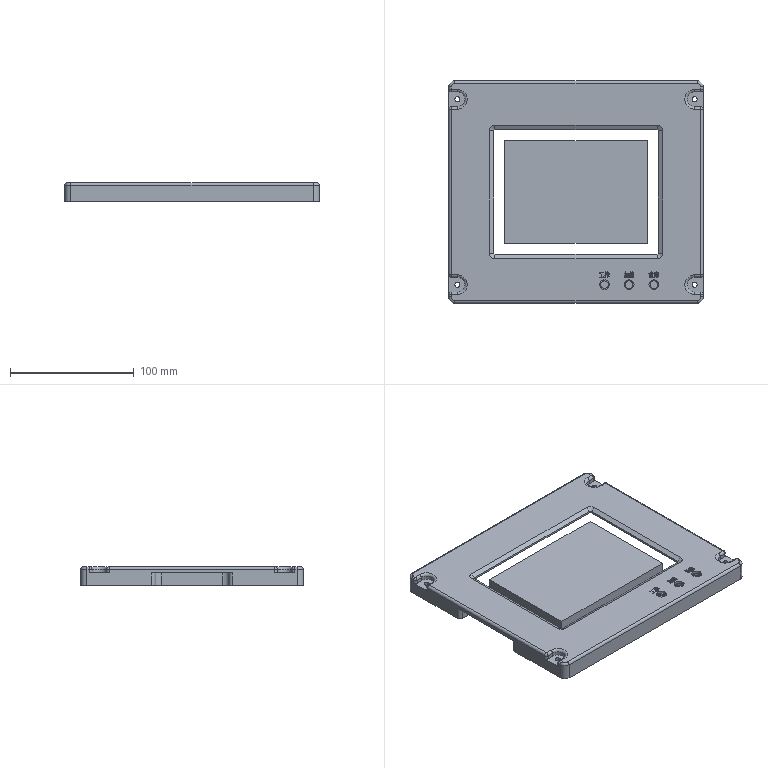NC program | Mastercam | posted with a generic post | part box 206 x 180 x 15 mm
Lines 17302 to 18142 of 42274:
(4 FEM |TOOL - 4|DIA. OFF. - 4|LEN. - 4|TOOL DIA. - 4.)
N4968 T4 M6
N4970 G0 G54 G90 X23. Y-75. C0. B0. S10000 M3
N4972 G43 H4 Z50.
N4974 Z1.
N4976 G1 Z0. F600.
N4978 X21.695 Y-74.65 F3000.
N4980 G3 X21.217 Y-75.478 I.478 J-.828
N4982 X21.346 Y-75.955 I.956
N4984 X23. Y-76.91 Z-.05 I1.654 J.955
N4986 X24.91 Y-75. Z-.125 J1.91
N4988 X23. Y-73.09 Z-.2 I-1.91
N4990 X21.09 Y-75. Z-.275 J-1.91
N4992 X21.346 Y-75.955 Z-.3 I1.91
N4994 X23. Y-76.91 Z-.35 I1.654 J.955
N4996 X24.91 Y-75. Z-.425 J1.91
N4998 X23. Y-73.09 Z-.5 I-1.91
N5000 X21.09 Y-75. Z-.575 J-1.91
N5002 X21.346 Y-75.955 Z-.6 I1.91
N5004 X23. Y-76.91 Z-.65 I1.654 J.955
N5006 X24.91 Y-75. Z-.725 J1.91
N5008 X23. Y-73.09 Z-.8 I-1.91
N5010 X21.09 Y-75. Z-.875 J-1.91
N5012 X21.346 Y-75.955 Z-.9 I1.91
N5014 X23. Y-76.91 Z-.95 I1.654 J.955
N5016 X24.91 Y-75. Z-1.025 J1.91
N5018 X23. Y-73.09 Z-1.1 I-1.91
N5020 X21.09 Y-75. Z-1.175 J-1.91
N5022 X21.346 Y-75.955 Z-1.2 I1.91
N5024 X23. Y-76.91 Z-1.25 I1.654 J.955
N5026 X24.91 Y-75. Z-1.325 J1.91
N5028 X23. Y-73.09 Z-1.4 I-1.91
N5030 X21.09 Y-75. Z-1.475 J-1.91
N5032 X21.346 Y-75.955 Z-1.5 I1.91
N5034 X23. Y-76.91 Z-1.55 I1.654 J.955
N5036 X24.91 Y-75. Z-1.625 J1.91
N5038 X23. Y-73.09 Z-1.7 I-1.91
N5040 X21.09 Y-75. Z-1.775 J-1.91
N5042 X21.346 Y-75.955 Z-1.8 I1.91
N5044 X23. Y-76.91 Z-1.85 I1.654 J.955
N5046 X24.91 Y-75. Z-1.925 J1.91
N5048 X23. Y-73.09 Z-2. I-1.91
N5050 X21.09 Y-75. J-1.91 F1500.
N5052 X23. Y-76.91 I1.91
N5054 X24.91 Y-75. J1.91
N5056 X23. Y-73.09 I-1.91
N5058 X22.506 Y-73.155 J-1.91
N5060 X21.798 Y-74.078 I.247 J-.923
N5062 X21.83 Y-74.325 I.955
N5064 G1 X23. Y-75.
N5066 G0 Z0.
N5068 G1 X24.005 Y-73.995 F750.
N5070 G3 X23. Y-72.99 I-1.005
N5072 X20.99 Y-75. J-2.01
N5074 X23. Y-77.01 I2.01
N5076 X25.01 Y-75. J2.01
N5078 X23. Y-72.99 I-2.01
N5080 X22.505 Y-73.052 J-2.01
N5082 X20.99 Y-75. Z-.631 I.495 J-1.948
N5084 X23. Y-77.01 Z-1.381 I2.01
N5086 X24.935 Y-75.546 Z-2. J2.01
N5088 X25.011 Y-75. I-1.935 J.546
N5090 X23. Y-72.989 I-2.011
N5092 X20.989 Y-75. J-2.011
N5094 X23. Y-77.011 I2.011
N5096 X24.935 Y-75.546 J2.011
N5098 X25.009 Y-75.052 I-1.935 J.546
N5100 G1 Y-75.026
N5102 G3 X24.031 Y-74.022 I-1.004
N5104 G1 X23. Y-75.
N5106 G0 Z50.
N5108 Z48.
N5110 Z-1.
N5112 G1 Z-2. F600.
N5114 X23.505 Y-74.495 F3000.
N5116 G3 X23. Y-73.99 I-.505
N5118 X21.99 Y-75. Z-2.075 J-1.01
N5120 X23. Y-76.01 Z-2.15 I1.01
N5122 X24.01 Y-75. Z-2.225 J1.01
N5124 X23. Y-73.99 Z-2.3 I-1.01
N5126 X21.99 Y-75. Z-2.375 J-1.01
N5128 X23. Y-76.01 Z-2.45 I1.01
N5130 X24.01 Y-75. Z-2.525 J1.01
N5132 X23. Y-73.99 Z-2.6 I-1.01
N5134 X21.99 Y-75. Z-2.675 J-1.01
N5136 X23. Y-76.01 Z-2.75 I1.01
N5138 X24.01 Y-75. Z-2.825 J1.01
N5140 X23. Y-73.99 Z-2.9 I-1.01
N5142 X21.99 Y-75. Z-2.975 J-1.01
N5144 X23. Y-76.01 Z-3.05 I1.01
N5146 X24.01 Y-75. Z-3.125 J1.01
N5148 X23. Y-73.99 Z-3.2 I-1.01
N5150 X21.99 Y-75. Z-3.275 J-1.01
N5152 X23. Y-76.01 Z-3.35 I1.01
N5154 X24.01 Y-75. Z-3.425 J1.01
N5156 X23. Y-73.99 Z-3.5 I-1.01
N5158 X21.99 Y-75. J-1.01 F1500.
N5160 X23. Y-76.01 I1.01
N5162 X24.01 Y-75. J1.01
N5164 X23. Y-73.99 I-1.01
N5166 X22.52 Y-74.111 J-1.01
N5168 X22.254 Y-74.556 I.24 J-.445
N5170 X22.316 Y-74.796 I.506
N5172 G1 X23. Y-75.
N5174 G0 Z-2.
N5176 G1 X23.555 Y-74.445 F750.
N5178 G3 X23. Y-73.89 I-.555
N5180 X21.89 Y-75. J-1.11
N5182 X23. Y-76.11 I1.11
N5184 X24.11 Y-75. J1.11
N5186 X23. Y-73.89 I-1.11
N5188 X22.517 Y-74.001 J-1.11
N5190 X21.89 Y-75. Z-2.535 I.483 J-.999
N5192 X23. Y-76.11 Z-3.285 I1.11
N5194 X23.483 Y-75.999 Z-3.5 J1.11
N5196 X24.11 Y-75. I-.483 J.999
N5198 X23. Y-73.89 I-1.11
N5200 X21.89 Y-75. J-1.11
N5202 X23. Y-76.11 I1.11
N5204 X23.483 Y-75.999 J1.11
N5206 X23.87 Y-75.689 I-.483 J.999
N5208 X23.99 Y-75.345 I-.435 J.344
N5210 X23.78 Y-74.91 I-.555
N5212 G1 X23. Y-75.
N5214 G0 Z48.
N5216 Z50.
N5218 X43.
N5220 Z1.
N5222 G1 Z0. F600.
N5224 X41.695 Y-74.65 F3000.
N5226 G3 X41.217 Y-75.478 I.478 J-.828
N5228 X41.346 Y-75.955 I.956
N5230 X43. Y-76.91 Z-.05 I1.654 J.955
N5232 X44.91 Y-75. Z-.125 J1.91
N5234 X43. Y-73.09 Z-.2 I-1.91
N5236 X41.09 Y-75. Z-.275 J-1.91
N5238 X41.346 Y-75.955 Z-.3 I1.91
N5240 X43. Y-76.91 Z-.35 I1.654 J.955
N5242 X44.91 Y-75. Z-.425 J1.91
N5244 X43. Y-73.09 Z-.5 I-1.91
N5246 X41.09 Y-75. Z-.575 J-1.91
N5248 X41.346 Y-75.955 Z-.6 I1.91
N5250 X43. Y-76.91 Z-.65 I1.654 J.955
N5252 X44.91 Y-75. Z-.725 J1.91
N5254 X43. Y-73.09 Z-.8 I-1.91
N5256 X41.09 Y-75. Z-.875 J-1.91
N5258 X41.346 Y-75.955 Z-.9 I1.91
N5260 X43. Y-76.91 Z-.95 I1.654 J.955
N5262 X44.91 Y-75. Z-1.025 J1.91
N5264 X43. Y-73.09 Z-1.1 I-1.91
N5266 X41.09 Y-75. Z-1.175 J-1.91
N5268 X41.346 Y-75.955 Z-1.2 I1.91
N5270 X43. Y-76.91 Z-1.25 I1.654 J.955
N5272 X44.91 Y-75. Z-1.325 J1.91
N5274 X43. Y-73.09 Z-1.4 I-1.91
N5276 X41.09 Y-75. Z-1.475 J-1.91
N5278 X41.346 Y-75.955 Z-1.5 I1.91
N5280 X43. Y-76.91 Z-1.55 I1.654 J.955
N5282 X44.91 Y-75. Z-1.625 J1.91
N5284 X43. Y-73.09 Z-1.7 I-1.91
N5286 X41.09 Y-75. Z-1.775 J-1.91
N5288 X41.346 Y-75.955 Z-1.8 I1.91
N5290 X43. Y-76.91 Z-1.85 I1.654 J.955
N5292 X44.91 Y-75. Z-1.925 J1.91
N5294 X43. Y-73.09 Z-2. I-1.91
N5296 X41.09 Y-75. J-1.91 F1500.
N5298 X43. Y-76.91 I1.91
N5300 X44.91 Y-75. J1.91
N5302 X43. Y-73.09 I-1.91
N5304 X42.506 Y-73.155 J-1.91
N5306 X41.798 Y-74.078 I.247 J-.923
N5308 X41.83 Y-74.325 I.955
N5310 G1 X43. Y-75.
N5312 G0 Z0.
N5314 G1 X44.005 Y-73.995 F750.
N5316 G3 X43. Y-72.99 I-1.005
N5318 X40.99 Y-75. J-2.01
N5320 X43. Y-77.01 I2.01
N5322 X45.01 Y-75. J2.01
N5324 X43. Y-72.99 I-2.01
N5326 X42.505 Y-73.052 J-2.01
N5328 X40.99 Y-75. Z-.631 I.495 J-1.948
N5330 X43. Y-77.01 Z-1.381 I2.01
N5332 X44.935 Y-75.546 Z-2. J2.01
N5334 X45.011 Y-75. I-1.935 J.546
N5336 X43. Y-72.989 I-2.011
N5338 X40.989 Y-75. J-2.011
N5340 X43. Y-77.011 I2.011
N5342 X44.935 Y-75.546 J2.011
N5344 X45.009 Y-75.052 I-1.935 J.546
N5346 G1 Y-75.026
N5348 G3 X44.031 Y-74.022 I-1.004
N5350 G1 X43. Y-75.
N5352 G0 Z50.
N5354 Z48.
N5356 Z-1.
N5358 G1 Z-2. F600.
N5360 X43.505 Y-74.495 F3000.
N5362 G3 X43. Y-73.99 I-.505
N5364 X41.99 Y-75. Z-2.075 J-1.01
N5366 X43. Y-76.01 Z-2.15 I1.01
N5368 X44.01 Y-75. Z-2.225 J1.01
N5370 X43. Y-73.99 Z-2.3 I-1.01
N5372 X41.99 Y-75. Z-2.375 J-1.01
N5374 X43. Y-76.01 Z-2.45 I1.01
N5376 X44.01 Y-75. Z-2.525 J1.01
N5378 X43. Y-73.99 Z-2.6 I-1.01
N5380 X41.99 Y-75. Z-2.675 J-1.01
N5382 X43. Y-76.01 Z-2.75 I1.01
N5384 X44.01 Y-75. Z-2.825 J1.01
N5386 X43. Y-73.99 Z-2.9 I-1.01
N5388 X41.99 Y-75. Z-2.975 J-1.01
N5390 X43. Y-76.01 Z-3.05 I1.01
N5392 X44.01 Y-75. Z-3.125 J1.01
N5394 X43. Y-73.99 Z-3.2 I-1.01
N5396 X41.99 Y-75. Z-3.275 J-1.01
N5398 X43. Y-76.01 Z-3.35 I1.01
N5400 X44.01 Y-75. Z-3.425 J1.01
N5402 X43. Y-73.99 Z-3.5 I-1.01
N5404 X41.99 Y-75. J-1.01 F1500.
N5406 X43. Y-76.01 I1.01
N5408 X44.01 Y-75. J1.01
N5410 X43. Y-73.99 I-1.01
N5412 X42.52 Y-74.111 J-1.01
N5414 X42.254 Y-74.556 I.24 J-.445
N5416 X42.316 Y-74.796 I.506
N5418 G1 X43. Y-75.
N5420 G0 Z-2.
N5422 G1 X43.555 Y-74.445 F750.
N5424 G3 X43. Y-73.89 I-.555
N5426 X41.89 Y-75. J-1.11
N5428 X43. Y-76.11 I1.11
N5430 X44.11 Y-75. J1.11
N5432 X43. Y-73.89 I-1.11
N5434 X42.517 Y-74.001 J-1.11
N5436 X41.89 Y-75. Z-2.535 I.483 J-.999
N5438 X43. Y-76.11 Z-3.285 I1.11
N5440 X43.483 Y-75.999 Z-3.5 J1.11
N5442 X44.11 Y-75. I-.483 J.999
N5444 X43. Y-73.89 I-1.11
N5446 X41.89 Y-75. J-1.11
N5448 X43. Y-76.11 I1.11
N5450 X43.483 Y-75.999 J1.11
N5452 X43.87 Y-75.689 I-.483 J.999
N5454 X43.99 Y-75.345 I-.435 J.344
N5456 X43.78 Y-74.91 I-.555
N5458 G1 X43. Y-75.
N5460 G0 Z48.
N5462 Z50.
N5464 X63.
N5466 Z1.
N5468 G1 Z0. F600.
N5470 X61.695 Y-74.65 F3000.
N5472 G3 X61.217 Y-75.478 I.478 J-.828
N5474 X61.346 Y-75.955 I.956
N5476 X63. Y-76.91 Z-.05 I1.654 J.955
N5478 X64.91 Y-75. Z-.125 J1.91
N5480 X63. Y-73.09 Z-.2 I-1.91
N5482 X61.09 Y-75. Z-.275 J-1.91
N5484 X61.346 Y-75.955 Z-.3 I1.91
N5486 X63. Y-76.91 Z-.35 I1.654 J.955
N5488 X64.91 Y-75. Z-.425 J1.91
N5490 X63. Y-73.09 Z-.5 I-1.91
N5492 X61.09 Y-75. Z-.575 J-1.91
N5494 X61.346 Y-75.955 Z-.6 I1.91
N5496 X63. Y-76.91 Z-.65 I1.654 J.955
N5498 X64.91 Y-75. Z-.725 J1.91
N5500 X63. Y-73.09 Z-.8 I-1.91
N5502 X61.09 Y-75. Z-.875 J-1.91
N5504 X61.346 Y-75.955 Z-.9 I1.91
N5506 X63. Y-76.91 Z-.95 I1.654 J.955
N5508 X64.91 Y-75. Z-1.025 J1.91
N5510 X63. Y-73.09 Z-1.1 I-1.91
N5512 X61.09 Y-75. Z-1.175 J-1.91
N5514 X61.346 Y-75.955 Z-1.2 I1.91
N5516 X63. Y-76.91 Z-1.25 I1.654 J.955
N5518 X64.91 Y-75. Z-1.325 J1.91
N5520 X63. Y-73.09 Z-1.4 I-1.91
N5522 X61.09 Y-75. Z-1.475 J-1.91
N5524 X61.346 Y-75.955 Z-1.5 I1.91
N5526 X63. Y-76.91 Z-1.55 I1.654 J.955
N5528 X64.91 Y-75. Z-1.625 J1.91
N5530 X63. Y-73.09 Z-1.7 I-1.91
N5532 X61.09 Y-75. Z-1.775 J-1.91
N5534 X61.346 Y-75.955 Z-1.8 I1.91
N5536 X63. Y-76.91 Z-1.85 I1.654 J.955
N5538 X64.91 Y-75. Z-1.925 J1.91
N5540 X63. Y-73.09 Z-2. I-1.91
N5542 X61.09 Y-75. J-1.91 F1500.
N5544 X63. Y-76.91 I1.91
N5546 X64.91 Y-75. J1.91
N5548 X63. Y-73.09 I-1.91
N5550 X62.506 Y-73.155 J-1.91
N5552 X61.798 Y-74.078 I.247 J-.923
N5554 X61.83 Y-74.325 I.955
N5556 G1 X63. Y-75.
N5558 G0 Z0.
N5560 G1 X64.005 Y-73.995 F750.
N5562 G3 X63. Y-72.99 I-1.005
N5564 X60.99 Y-75. J-2.01
N5566 X63. Y-77.01 I2.01
N5568 X65.01 Y-75. J2.01
N5570 X63. Y-72.99 I-2.01
N5572 X62.505 Y-73.052 J-2.01
N5574 X60.99 Y-75. Z-.631 I.495 J-1.948
N5576 X63. Y-77.01 Z-1.381 I2.01
N5578 X64.935 Y-75.546 Z-2. J2.01
N5580 X65.011 Y-75. I-1.935 J.546
N5582 X63. Y-72.989 I-2.011
N5584 X60.989 Y-75. J-2.011
N5586 X63. Y-77.011 I2.011
N5588 X64.935 Y-75.546 J2.011
N5590 X65.009 Y-75.052 I-1.935 J.546
N5592 G1 Y-75.026
N5594 G3 X64.031 Y-74.022 I-1.004
N5596 G1 X63. Y-75.
N5598 G0 Z50.
N5600 Z48.
N5602 Z-1.
N5604 G1 Z-2. F600.
N5606 X63.505 Y-74.495 F3000.
N5608 G3 X63. Y-73.99 I-.505
N5610 X61.99 Y-75. Z-2.075 J-1.01
N5612 X63. Y-76.01 Z-2.15 I1.01
N5614 X64.01 Y-75. Z-2.225 J1.01
N5616 X63. Y-73.99 Z-2.3 I-1.01
N5618 X61.99 Y-75. Z-2.375 J-1.01
N5620 X63. Y-76.01 Z-2.45 I1.01
N5622 X64.01 Y-75. Z-2.525 J1.01
N5624 X63. Y-73.99 Z-2.6 I-1.01
N5626 X61.99 Y-75. Z-2.675 J-1.01
N5628 X63. Y-76.01 Z-2.75 I1.01
N5630 X64.01 Y-75. Z-2.825 J1.01
N5632 X63. Y-73.99 Z-2.9 I-1.01
N5634 X61.99 Y-75. Z-2.975 J-1.01
N5636 X63. Y-76.01 Z-3.05 I1.01
N5638 X64.01 Y-75. Z-3.125 J1.01
N5640 X63. Y-73.99 Z-3.2 I-1.01
N5642 X61.99 Y-75. Z-3.275 J-1.01
N5644 X63. Y-76.01 Z-3.35 I1.01
N5646 X64.01 Y-75. Z-3.425 J1.01
N5648 X63. Y-73.99 Z-3.5 I-1.01
N5650 X61.99 Y-75. J-1.01 F1500.
N5652 X63. Y-76.01 I1.01
N5654 X64.01 Y-75. J1.01
N5656 X63. Y-73.99 I-1.01
N5658 X62.52 Y-74.111 J-1.01
N5660 X62.254 Y-74.556 I.24 J-.445
N5662 X62.316 Y-74.796 I.506
N5664 G1 X63. Y-75.
N5666 G0 Z-2.
N5668 G1 X63.555 Y-74.445 F750.
N5670 G3 X63. Y-73.89 I-.555
N5672 X61.89 Y-75. J-1.11
N5674 X63. Y-76.11 I1.11
N5676 X64.11 Y-75. J1.11
N5678 X63. Y-73.89 I-1.11
N5680 X62.517 Y-74.001 J-1.11
N5682 X61.89 Y-75. Z-2.535 I.483 J-.999
N5684 X63. Y-76.11 Z-3.285 I1.11
N5686 X63.483 Y-75.999 Z-3.5 J1.11
N5688 X64.11 Y-75. I-.483 J.999
N5690 X63. Y-73.89 I-1.11
N5692 X61.89 Y-75. J-1.11
N5694 X63. Y-76.11 I1.11
N5696 X63.483 Y-75.999 J1.11
N5698 X63.87 Y-75.689 I-.483 J.999
N5700 X63.99 Y-75.345 I-.435 J.344
N5702 X63.78 Y-74.91 I-.555
N5704 G1 X63. Y-75.
N5706 G0 Z48.
N5708 M5
N5710 G0 G28 G91 Z0.
N5712 G28
N5714 M01
N5716 G0 G17 G40 G80 G90 G94 G98
N5718 G0 G28 G91 Z0.
(8 FEM |TOOL - 8|DIA. OFF. - 8|LEN. - 8|TOOL DIA. - 8.)
N5720 T8 M6
N5722 G0 G54 G90 X-44.1 Y-.8 C0. B0. S7000 M3
N5724 G43 H8 Z50.
N5726 Z1.
N5728 G1 Z0. F600.
N5730 X-43.3 F3000.
N5732 G3 X-42.5 Y0. J.8
N5734 X-45. Y2.5 Z-.1 I-2.5
N5736 X-47.5 Y0. Z-.2 J-2.5
N5738 X-45. Y-2.5 Z-.3 I2.5
N5740 X-42.5 Y0. Z-.4 J2.5
N5742 X-45. Y2.5 Z-.5 I-2.5
N5744 X-47.5 Y0. Z-.6 J-2.5
N5746 X-45. Y-2.5 Z-.7 I2.5
N5748 X-42.5 Y0. Z-.8 J2.5
N5750 X-45. Y2.5 Z-.9 I-2.5
N5752 X-47.5 Y0. Z-1. J-2.5
N5754 X-45. Y-2.5 Z-1.1 I2.5
N5756 X-42.5 Y0. Z-1.2 J2.5
N5758 X-45. Y2.5 Z-1.3 I-2.5
N5760 X-47.5 Y0. Z-1.4 J-2.5
N5762 X-45. Y-2.5 Z-1.5 I2.5
N5764 X-42.5 Y0. Z-1.6 J2.5
N5766 X-45. Y2.5 Z-1.7 I-2.5
N5768 X-47.5 Y0. Z-1.8 J-2.5
N5770 X-45. Y-2.5 Z-1.9 I2.5
N5772 X-42.5 Y0. Z-2. J2.5
N5774 X-45. Y2.5 Z-2.1 I-2.5
N5776 X-47.5 Y0. Z-2.2 J-2.5
N5778 X-45. Y-2.5 Z-2.3 I2.5
N5780 X-42.5 Y0. Z-2.4 J2.5
N5782 X-45. Y2.5 Z-2.5 I-2.5
N5784 X-47.5 Y0. Z-2.6 J-2.5
N5786 X-45. Y-2.5 Z-2.7 I2.5
N5788 X-42.5 Y0. Z-2.8 J2.5
N5790 X-45. Y2.5 Z-2.9 I-2.5
N5792 X-47.5 Y0. Z-3. J-2.5
N5794 X-45. Y-2.5 Z-3.1 I2.5
N5796 X-42.5 Y0. Z-3.2 J2.5
N5798 X-45. Y2.5 Z-3.3 I-2.5
N5800 X-47.5 Y0. Z-3.4 J-2.5
N5802 X-45. Y-2.5 Z-3.5 I2.5
N5804 X-42.5 Y0. Z-3.6 J2.5
N5806 X-45. Y2.5 Z-3.7 I-2.5
N5808 X-47.5 Y0. Z-3.8 J-2.5
N5810 X-45. Y-2.5 Z-3.9 I2.5
N5812 X-42.5 Y0. Z-4. J2.5
N5814 X-45. Y2.5 Z-4.1 I-2.5
N5816 X-47.5 Y0. Z-4.2 J-2.5
N5818 X-45. Y-2.5 Z-4.3 I2.5
N5820 X-42.5 Y0. Z-4.4 J2.5
N5822 X-45. Y2.5 Z-4.5 I-2.5
N5824 X-47.5 Y0. Z-4.6 J-2.5
N5826 X-45. Y-2.5 Z-4.7 I2.5
N5828 X-42.5 Y0. Z-4.8 J2.5
N5830 X-45. Y2.5 Z-4.9 I-2.5
N5832 X-47.5 Y0. Z-5. J-2.5
N5834 X-45. Y-2.5 Z-5.1 I2.5
N5836 X-42.5 Y0. Z-5.2 J2.5
N5838 X-45. Y2.5 Z-5.3 I-2.5
N5840 X-47.5 Y0. Z-5.4 J-2.5
N5842 X-45. Y-2.5 Z-5.5 I2.5
N5844 X-42.5 Y0. Z-5.6 J2.5
N5846 X-45. Y2.5 Z-5.7 I-2.5
N5848 X-47.5 Y0. Z-5.8 J-2.5
N5850 X-45. Y-2.5 Z-5.9 I2.5
N5852 X-42.5 Y0. Z-6. J2.5
N5854 X-45. Y2.5 Z-6.1 I-2.5
N5856 X-47.5 Y0. Z-6.2 J-2.5
N5858 X-45. Y-2.5 Z-6.3 I2.5
N5860 X-42.5 Y0. Z-6.4 J2.5
N5862 X-45. Y2.5 Z-6.5 I-2.5
N5864 X-47.5 Y0. Z-6.6 J-2.5
N5866 X-45. Y-2.5 Z-6.7 I2.5
N5868 X-42.5 Y0. Z-6.8 J2.5
N5870 X-45. Y2.5 Z-6.9 I-2.5
N5872 X-47.5 Y0. Z-7. J-2.5
N5874 X-45. Y-2.5 Z-7.1 I2.5
N5876 X-42.5 Y0. Z-7.2 J2.5
N5878 X-45. Y2.5 Z-7.3 I-2.5
N5880 X-47.5 Y0. Z-7.4 J-2.5
N5882 X-45. Y-2.5 Z-7.5 I2.5
N5884 X-42.5 Y0. Z-7.6 J2.5
N5886 X-45. Y2.5 Z-7.7 I-2.5
N5888 X-47.5 Y0. Z-7.8 J-2.5
N5890 X-45. Y-2.5 Z-7.9 I2.5
N5892 X-42.5 Y0. Z-8. J2.5
N5894 X-45. Y2.5 Z-8.1 I-2.5
N5896 X-47.5 Y0. Z-8.2 J-2.5
N5898 X-45. Y-2.5 Z-8.3 I2.5
N5900 X-42.5 Y0. Z-8.4 J2.5
N5902 X-45. Y2.5 Z-8.5 I-2.5
N5904 X-47.5 Y0. Z-8.6 J-2.5
N5906 X-45. Y-2.5 Z-8.7 I2.5
N5908 X-42.5 Y0. Z-8.8 J2.5
N5910 X-45. Y2.5 Z-8.9 I-2.5
N5912 X-47.5 Y0. Z-9. J-2.5
N5914 X-45. Y-2.5 Z-9.1 I2.5
N5916 X-42.5 Y0. Z-9.2 J2.5
N5918 X-45. Y2.5 Z-9.3 I-2.5
N5920 X-47.5 Y0. Z-9.4 J-2.5
N5922 X-45. Y-2.5 Z-9.5 I2.5
N5924 X-42.5 Y0. Z-9.6 J2.5
N5926 X-45. Y2.5 Z-9.7 I-2.5
N5928 X-47.5 Y0. Z-9.8 J-2.5
N5930 X-45. Y-2.5 Z-9.9 I2.5
N5932 X-42.5 Y0. Z-10. J2.5
N5934 X-45. Y2.5 Z-10.1 I-2.5
N5936 X-47.5 Y0. Z-10.2 J-2.5
N5938 X-45. Y-2.5 Z-10.3 I2.5
N5940 X-42.5 Y0. Z-10.4 J2.5
N5942 X-45. Y2.5 Z-10.5 I-2.5
N5944 X-47.5 Y0. Z-10.6 J-2.5
N5946 X-45. Y-2.5 Z-10.7 I2.5
N5948 X-42.5 Y0. Z-10.8 J2.5
N5950 X-45. Y2.5 Z-10.9 I-2.5
N5952 X-47.5 Y0. Z-11. J-2.5
N5954 X-45. Y-2.5 Z-11.1 I2.5
N5956 X-42.5 Y0. Z-11.2 J2.5
N5958 X-45. Y2.5 Z-11.3 I-2.5
N5960 X-47.5 Y0. Z-11.4 J-2.5
N5962 X-45. Y-2.5 Z-11.5 I2.5
N5964 X-42.5 Y0. Z-11.6 J2.5
N5966 X-45. Y2.5 Z-11.7 I-2.5
N5968 X-47.5 Y0. Z-11.8 J-2.5
N5970 X-45. Y-2.5 Z-11.9 I2.5
N5972 X-42.5 Y0. Z-12. J2.5
N5974 X-45. Y2.5 Z-12.1 I-2.5
N5976 X-47.5 Y0. Z-12.2 J-2.5
N5978 X-45. Y-2.5 Z-12.3 I2.5
N5980 X-42.5 Y0. Z-12.4 J2.5
N5982 X-45. Y2.5 Z-12.5 I-2.5
N5984 X-47.5 Y0. Z-12.6 J-2.5
N5986 X-45. Y-2.5 Z-12.7 I2.5
N5988 X-42.5 Y0. Z-12.8 J2.5
N5990 X-45. Y2.5 Z-12.9 I-2.5
N5992 X-47.5 Y0. Z-13. J-2.5
N5994 X-45. Y-2.5 Z-13.1 I2.5
N5996 X-42.5 Y0. Z-13.2 J2.5
N5998 X-45. Y2.5 Z-13.3 I-2.5
N6000 X-47.5 Y0. Z-13.4 J-2.5
N6002 X-45. Y-2.5 Z-13.5 I2.5
N6004 X-42.5 Y0. Z-13.6 J2.5
N6006 X-45. Y2.5 Z-13.7 I-2.5
N6008 X-47.5 Y0. Z-13.8 J-2.5
N6010 X-45. Y-2.5 Z-13.9 I2.5
N6012 X-42.5 Y0. Z-14. J2.5
N6014 X-45. Y2.5 Z-14.1 I-2.5
N6016 X-47.5 Y0. Z-14.2 J-2.5
N6018 X-45. Y-2.5 Z-14.3 I2.5
N6020 X-42.5 Y0. Z-14.4 J2.5
N6022 X-45. Y2.5 Z-14.5 I-2.5
N6024 X-47.5 Y0. Z-14.6 J-2.5
N6026 X-45. Y-2.5 Z-14.7 I2.5
N6028 X-42.5 Y0. Z-14.8 J2.5
N6030 X-45. Y2.5 Z-14.9 I-2.5
N6032 X-47.5 Y0. J-2.5
N6034 X-45. Y-2.5 I2.5
N6036 X-42.5 Y0. J2.5
N6038 X-45. Y2.5 I-2.5
N6040 X-45.8 Y1.7 J-.8
N6042 G1 Y.9
N6044 G0 Z50.
N6046 X45.9 Y-.8
N6048 Z1.
N6050 G1 Z0. F600.
N6052 X46.7 F3000.
N6054 G3 X47.5 Y0. J.8
N6056 X45. Y2.5 Z-.1 I-2.5
N6058 X42.5 Y0. Z-.2 J-2.5
N6060 X45. Y-2.5 Z-.3 I2.5
N6062 X47.5 Y0. Z-.4 J2.5
N6064 X45. Y2.5 Z-.5 I-2.5
N6066 X42.5 Y0. Z-.6 J-2.5
N6068 X45. Y-2.5 Z-.7 I2.5
N6070 X47.5 Y0. Z-.8 J2.5
N6072 X45. Y2.5 Z-.9 I-2.5
N6074 X42.5 Y0. Z-1. J-2.5
N6076 X45. Y-2.5 Z-1.1 I2.5
N6078 X47.5 Y0. Z-1.2 J2.5
N6080 X45. Y2.5 Z-1.3 I-2.5
N6082 X42.5 Y0. Z-1.4 J-2.5
N6084 X45. Y-2.5 Z-1.5 I2.5
N6086 X47.5 Y0. Z-1.6 J2.5
N6088 X45. Y2.5 Z-1.7 I-2.5
N6090 X42.5 Y0. Z-1.8 J-2.5
N6092 X45. Y-2.5 Z-1.9 I2.5
N6094 X47.5 Y0. Z-2. J2.5
N6096 X45. Y2.5 Z-2.1 I-2.5
N6098 X42.5 Y0. Z-2.2 J-2.5
N6100 X45. Y-2.5 Z-2.3 I2.5
N6102 X47.5 Y0. Z-2.4 J2.5
N6104 X45. Y2.5 Z-2.5 I-2.5
N6106 X42.5 Y0. Z-2.6 J-2.5
N6108 X45. Y-2.5 Z-2.7 I2.5
N6110 X47.5 Y0. Z-2.8 J2.5
N6112 X45. Y2.5 Z-2.9 I-2.5
N6114 X42.5 Y0. Z-3. J-2.5
N6116 X45. Y-2.5 Z-3.1 I2.5
N6118 X47.5 Y0. Z-3.2 J2.5
N6120 X45. Y2.5 Z-3.3 I-2.5
N6122 X42.5 Y0. Z-3.4 J-2.5
N6124 X45. Y-2.5 Z-3.5 I2.5
N6126 X47.5 Y0. Z-3.6 J2.5
N6128 X45. Y2.5 Z-3.7 I-2.5
N6130 X42.5 Y0. Z-3.8 J-2.5
N6132 X45. Y-2.5 Z-3.9 I2.5
N6134 X47.5 Y0. Z-4. J2.5
N6136 X45. Y2.5 Z-4.1 I-2.5
N6138 X42.5 Y0. Z-4.2 J-2.5
N6140 X45. Y-2.5 Z-4.3 I2.5
N6142 X47.5 Y0. Z-4.4 J2.5
N6144 X45. Y2.5 Z-4.5 I-2.5
N6146 X42.5 Y0. Z-4.6 J-2.5
N6148 X45. Y-2.5 Z-4.7 I2.5
N6150 X47.5 Y0. Z-4.8 J2.5
N6152 X45. Y2.5 Z-4.9 I-2.5
N6154 X42.5 Y0. Z-5. J-2.5
N6156 X45. Y-2.5 Z-5.1 I2.5
N6158 X47.5 Y0. Z-5.2 J2.5
N6160 X45. Y2.5 Z-5.3 I-2.5
N6162 X42.5 Y0. Z-5.4 J-2.5
N6164 X45. Y-2.5 Z-5.5 I2.5
N6166 X47.5 Y0. Z-5.6 J2.5
N6168 X45. Y2.5 Z-5.7 I-2.5
N6170 X42.5 Y0. Z-5.8 J-2.5
N6172 X45. Y-2.5 Z-5.9 I2.5
N6174 X47.5 Y0. Z-6. J2.5
N6176 X45. Y2.5 Z-6.1 I-2.5
N6178 X42.5 Y0. Z-6.2 J-2.5
N6180 X45. Y-2.5 Z-6.3 I2.5
N6182 X47.5 Y0. Z-6.4 J2.5
N6184 X45. Y2.5 Z-6.5 I-2.5
N6186 X42.5 Y0. Z-6.6 J-2.5
N6188 X45. Y-2.5 Z-6.7 I2.5
N6190 X47.5 Y0. Z-6.8 J2.5
N6192 X45. Y2.5 Z-6.9 I-2.5
N6194 X42.5 Y0. Z-7. J-2.5
N6196 X45. Y-2.5 Z-7.1 I2.5
N6198 X47.5 Y0. Z-7.2 J2.5
N6200 X45. Y2.5 Z-7.3 I-2.5
N6202 X42.5 Y0. Z-7.4 J-2.5
N6204 X45. Y-2.5 Z-7.5 I2.5
N6206 X47.5 Y0. Z-7.6 J2.5
N6208 X45. Y2.5 Z-7.7 I-2.5
N6210 X42.5 Y0. Z-7.8 J-2.5
N6212 X45. Y-2.5 Z-7.9 I2.5
N6214 X47.5 Y0. Z-8. J2.5
N6216 X45. Y2.5 Z-8.1 I-2.5
N6218 X42.5 Y0. Z-8.2 J-2.5
N6220 X45. Y-2.5 Z-8.3 I2.5
N6222 X47.5 Y0. Z-8.4 J2.5
N6224 X45. Y2.5 Z-8.5 I-2.5
N6226 X42.5 Y0. Z-8.6 J-2.5
N6228 X45. Y-2.5 Z-8.7 I2.5
N6230 X47.5 Y0. Z-8.8 J2.5
N6232 X45. Y2.5 Z-8.9 I-2.5
N6234 X42.5 Y0. Z-9. J-2.5
N6236 X45. Y-2.5 Z-9.1 I2.5
N6238 X47.5 Y0. Z-9.2 J2.5
N6240 X45. Y2.5 Z-9.3 I-2.5
N6242 X42.5 Y0. Z-9.4 J-2.5
N6244 X45. Y-2.5 Z-9.5 I2.5
N6246 X47.5 Y0. Z-9.6 J2.5
N6248 X45. Y2.5 Z-9.7 I-2.5
N6250 X42.5 Y0. Z-9.8 J-2.5
N6252 X45. Y-2.5 Z-9.9 I2.5
N6254 X47.5 Y0. Z-10. J2.5
N6256 X45. Y2.5 Z-10.1 I-2.5
N6258 X42.5 Y0. Z-10.2 J-2.5
N6260 X45. Y-2.5 Z-10.3 I2.5
N6262 X47.5 Y0. Z-10.4 J2.5
N6264 X45. Y2.5 Z-10.5 I-2.5
N6266 X42.5 Y0. Z-10.6 J-2.5
N6268 X45. Y-2.5 Z-10.7 I2.5
N6270 X47.5 Y0. Z-10.8 J2.5
N6272 X45. Y2.5 Z-10.9 I-2.5
N6274 X42.5 Y0. Z-11. J-2.5
N6276 X45. Y-2.5 Z-11.1 I2.5
N6278 X47.5 Y0. Z-11.2 J2.5
N6280 X45. Y2.5 Z-11.3 I-2.5
N6282 X42.5 Y0. Z-11.4 J-2.5
N6284 X45. Y-2.5 Z-11.5 I2.5
N6286 X47.5 Y0. Z-11.6 J2.5
N6288 X45. Y2.5 Z-11.7 I-2.5
N6290 X42.5 Y0. Z-11.8 J-2.5
N6292 X45. Y-2.5 Z-11.9 I2.5
N6294 X47.5 Y0. Z-12. J2.5
N6296 X45. Y2.5 Z-12.1 I-2.5
N6298 X42.5 Y0. Z-12.2 J-2.5
N6300 X45. Y-2.5 Z-12.3 I2.5
N6302 X47.5 Y0. Z-12.4 J2.5
N6304 X45. Y2.5 Z-12.5 I-2.5
N6306 X42.5 Y0. Z-12.6 J-2.5
N6308 X45. Y-2.5 Z-12.7 I2.5
N6310 X47.5 Y0. Z-12.8 J2.5
N6312 X45. Y2.5 Z-12.9 I-2.5
N6314 X42.5 Y0. Z-13. J-2.5
N6316 X45. Y-2.5 Z-13.1 I2.5
N6318 X47.5 Y0. Z-13.2 J2.5
N6320 X45. Y2.5 Z-13.3 I-2.5
N6322 X42.5 Y0. Z-13.4 J-2.5
N6324 X45. Y-2.5 Z-13.5 I2.5
N6326 X47.5 Y0. Z-13.6 J2.5
N6328 X45. Y2.5 Z-13.7 I-2.5
N6330 X42.5 Y0. Z-13.8 J-2.5
N6332 X45. Y-2.5 Z-13.9 I2.5
N6334 X47.5 Y0. Z-14. J2.5
N6336 X45. Y2.5 Z-14.1 I-2.5
N6338 X42.5 Y0. Z-14.2 J-2.5
N6340 X45. Y-2.5 Z-14.3 I2.5
N6342 X47.5 Y0. Z-14.4 J2.5
N6344 X45. Y2.5 Z-14.5 I-2.5
N6346 X42.5 Y0. Z-14.6 J-2.5
N6348 X45. Y-2.5 Z-14.7 I2.5
N6350 X47.5 Y0. Z-14.8 J2.5
N6352 X45. Y2.5 Z-14.9 I-2.5
N6354 X42.5 Y0. J-2.5
N6356 X45. Y-2.5 I2.5
N6358 X47.5 Y0. J2.5
N6360 X45. Y2.5 I-2.5
N6362 X44.2 Y1.7 J-.8
N6364 G1 Y.9
N6366 G0 Z50.
N6368 M5
N6370 G0 G28 G91 Z0.
N6372 G28
N6374 M01
N6376 G0 G17 G40 G80 G90 G94 G98
N6378 G0 G28 G91 Z0.
(4 CHM |TOOL - 5|DIA. OFF. - 5|LEN. - 5|TOOL DIA. - 4.)
N6380 T5 M6
N6382 G0 G54 G90 X96. Y-75. C0. B0. S3000 M3
N6384 G43 H5 Z45.
N6386 G81 G98 Z-5.7 R-4. F300.
N6388 Y75.
N6390 X-96.
N6392 Y-75.
N6394 G80
N6396 S7000 M3
N6398 Z50.
N6400 X25.55 Y-75.4
N6402 Z1.
N6404 G1 Z-.7 F600.
N6406 X25.95 F1000.
N6408 G3 X26.35 Y-75. J.4
N6410 X23. Y-71.65 I-3.35
N6412 X19.65 Y-75. J-3.35
N6414 X23. Y-78.35 I3.35
N6416 X26.35 Y-75. J3.35
N6418 X25.95 Y-74.6 I-.4
N6420 G1 X25.55
N6422 G0 Z50.
N6424 X45.55 Y-75.4
N6426 Z1.
N6428 G1 Z-.7 F600.
N6430 X45.95 F1000.
N6432 G3 X46.35 Y-75. J.4
N6434 X43. Y-71.65 I-3.35
N6436 X39.65 Y-75. J-3.35
N6438 X43. Y-78.35 I3.35
N6440 X46.35 Y-75. J3.35
N6442 X45.95 Y-74.6 I-.4
N6444 G1 X45.55
N6446 G0 Z50.
N6448 X65.55 Y-75.4
N6450 Z1.
N6452 G1 Z-.7 F600.
N6454 X65.95 F1000.
N6456 G3 X66.35 Y-75. J.4
N6458 X63. Y-71.65 I-3.35
N6460 X59.65 Y-75. J-3.35
N6462 X63. Y-78.35 I3.35
N6464 X66.35 Y-75. J3.35
N6466 X65.95 Y-74.6 I-.4
N6468 G1 X65.55
N6470 G0 Z50.
N6472 X-39.95 Y-.4
N6474 Z1.
N6476 G1 Z-.7 F600.
N6478 X-39.55 F1000.
N6480 G3 X-39.15 Y0. J.4
N6482 X-45. Y5.85 I-5.85
N6484 X-50.85 Y0. J-5.85
N6486 X-45. Y-5.85 I5.85
N6488 X-39.15 Y0. J5.85
N6490 X-39.55 Y.4 I-.4
N6492 G1 X-39.95
N6494 G0 Z50.
N6496 X50.05 Y-.4
N6498 Z1.
N6500 G1 Z-.7 F600.
N6502 X50.45 F1000.
N6504 G3 X50.85 Y0. J.4
N6506 X45. Y5.85 I-5.85
N6508 X39.15 Y0. J-5.85
N6510 X45. Y-5.85 I5.85
N6512 X50.85 Y0. J5.85
N6514 X50.45 Y.4 I-.4
N6516 G1 X50.05
N6518 G0 Z50.
N6520 X24.15 Y-75.4
N6522 Z1.
N6524 G1 Z-3.2 F600.
N6526 X24.55 F1000.
N6528 G3 X24.95 Y-75. J.4
N6530 X23. Y-73.05 I-1.95
N6532 X21.05 Y-75. J-1.95
N6534 X23. Y-76.95 I1.95
N6536 X24.95 Y-75. J1.95
N6538 X24.55 Y-74.6 I-.4
N6540 G1 X24.15
N6542 G0 Z50.
N6544 X44.15 Y-75.4
N6546 Z1.
N6548 G1 Z-3.2 F600.
N6550 X44.55 F1000.
N6552 G3 X44.95 Y-75. J.4
N6554 X43. Y-73.05 I-1.95
N6556 X41.05 Y-75. J-1.95
N6558 X43. Y-76.95 I1.95
N6560 X44.95 Y-75. J1.95
N6562 X44.55 Y-74.6 I-.4
N6564 G1 X44.15
N6566 G0 Z50.
N6568 X64.15 Y-75.4
N6570 Z1.
N6572 G1 Z-3.2 F600.
N6574 X64.55 F1000.
N6576 G3 X64.95 Y-75. J.4
N6578 X63. Y-73.05 I-1.95
N6580 X61.05 Y-75. J-1.95
N6582 X63. Y-76.95 I1.95
N6584 X64.95 Y-75. J1.95
N6586 X64.55 Y-74.6 I-.4
N6588 G1 X64.15
N6590 G0 Z50.
N6592 M5
N6594 G0 G28 G91 Z0.
N6596 G28
N6598 M01
N6600 G0 G17 G40 G80 G90 G94 G98
N6602 G0 G28 G91 Z0.
(100 FEM |TOOL - 24|DIA. OFF. - 24|LEN. - 24|TOOL DIA. - 100.)
N6604 T24 M6
N6606 G0 G54 G90 X-215.5 Y64.998 C0. B0. S4000 M3
N6608 G43 H24 Z51.
N6610 Z3.
N6612 G1 Z0. F600.
N6614 X155.5 F1000.
N6616 G2 X187.999 Y32.499 J-32.499
N6618 X155.5 Y0. I-32.499
N6620 G1 X-155.5
N6622 G3 X-187.999 Y-32.499 J-32.499
N6624 X-155.5 Y-64.998 I32.499
N6626 G1 X215.5
N6628 G0 Z50.
N6630 M5
N6632 G0 G28 G91 Z0.
N6634 G28
N6636 M01
N6638 G0 G17 G40 G80 G90 G94 G98
N6640 G0 G28 G91 Z0.